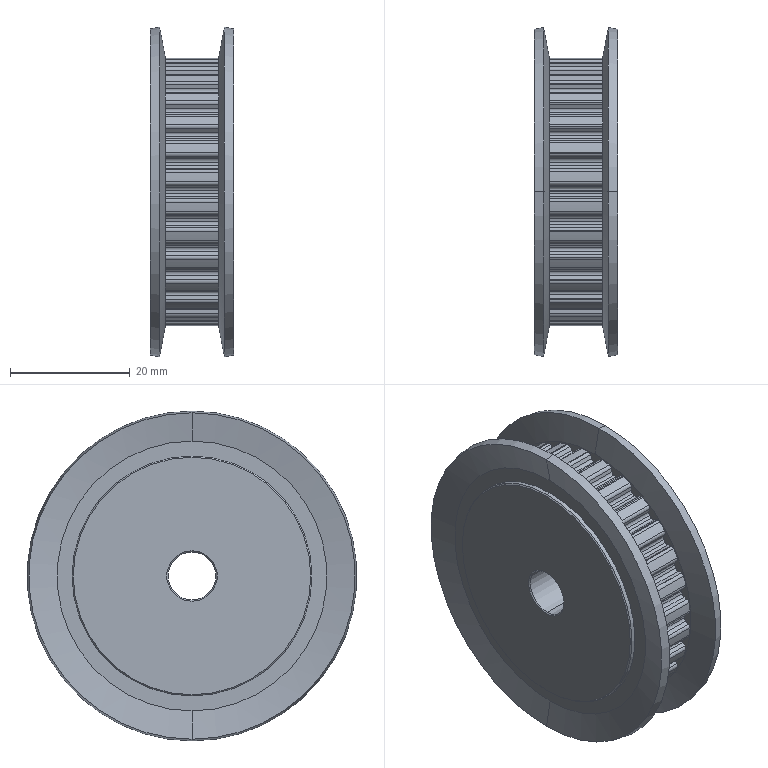Part | SolidWorks | features BaseBody 1 | 1 solid | 277 faces | box 14 x 55 x 55 mm | volume 22610 mm3 | cylinder 199 | plane 62 | cone 16 | commonest cylinder face diameters 1.22 x136 41.97 x29 44.77 x28 40 x4 8 x2